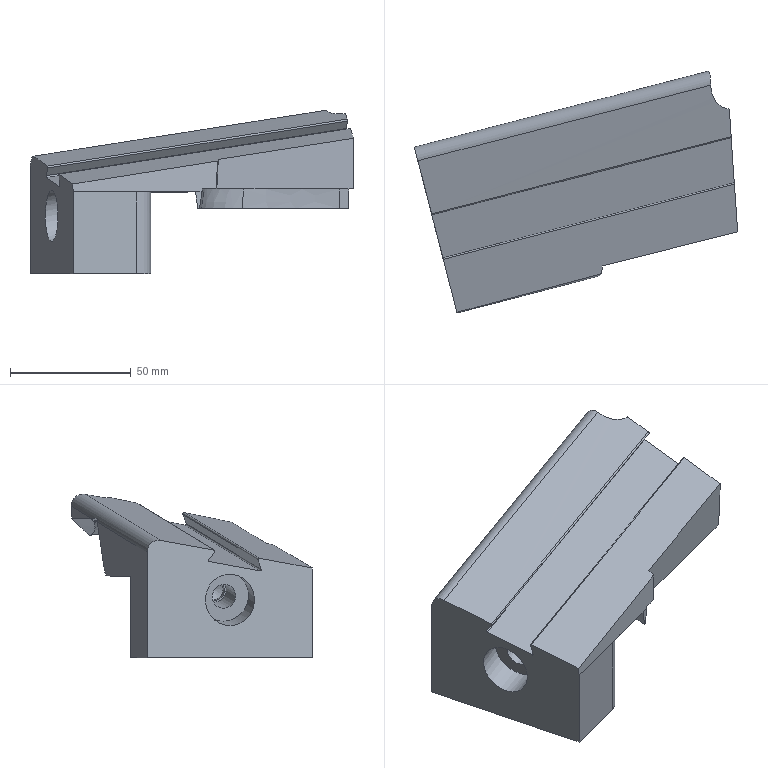Part | STEP file | 车灯-后视镜_id410_x_t | 1 solid | 116 faces | box 133.87 x 99.984 x 67.76 mm | volume 199506 mm3 | spline 45 | plane 41 | cylinder 19 | other 10 | cone 1 | commonest cylinder face diameters 1 x4 0.22 x3 10 x3 4 x2 6 x2 16 x2